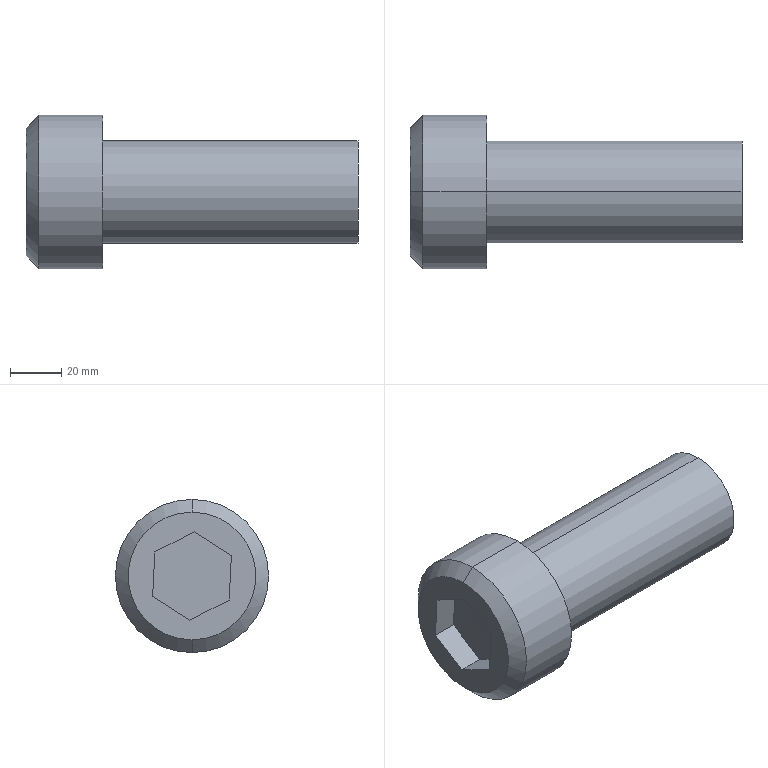Part | SolidWorks | features BaseBody 12, ICE 10, Chamfer 2 | 1 solid | 16 faces | box 130 x 60 x 60 mm | volume 200467 mm3 | plane 10 | cylinder 4 | cone 2 | commonest cylinder face diameters 40 x2 60 x2
STEP:
#1=CARTESIAN_POINT('',(548.124,-238.28,806.023));
#2=VERTEX_POINT('',#1);
#3=CARTESIAN_POINT('',(548.124,-238.28,846.023));
#4=VERTEX_POINT('',#3);
#5=CARTESIAN_POINT('',(548.124,-238.28,826.023));
#6=DIRECTION('',(1.,0.,0.));
#7=DIRECTION('',(0.,0.,-1.));
#8=AXIS2_PLACEMENT_3D('',#5,#6,#7);
#9=CIRCLE('',#8,20.);
#10=EDGE_CURVE('',#2,#4,#9,.T.);
#11=ORIENTED_EDGE('',*,*,#10,.F.);
#12=CARTESIAN_POINT('',(448.124,-238.28,806.023));
#13=VERTEX_POINT('',#12);
#14=CARTESIAN_POINT('',(548.124,-238.28,806.023));
#15=DIRECTION('',(-1.,0.,0.));
#16=VECTOR('',#15,1000.);
#17=LINE('',#14,#16);
#18=EDGE_CURVE('',#2,#13,#17,.T.);
#19=ORIENTED_EDGE('',*,*,#18,.T.);
#20=CARTESIAN_POINT('',(448.124,-238.28,846.023));
#21=VERTEX_POINT('',#20);
#22=CARTESIAN_POINT('',(448.124,-238.28,826.023));
#23=DIRECTION('',(1.,0.,0.));
#24=DIRECTION('',(0.,0.,-1.));
#25=AXIS2_PLACEMENT_3D('',#22,#23,#24);
#26=CIRCLE('',#25,20.);
#27=EDGE_CURVE('',#13,#21,#26,.T.);
#28=ORIENTED_EDGE('',*,*,#27,.T.);
#29=CARTESIAN_POINT('',(548.124,-238.28,846.023));
#30=DIRECTION('',(-1.,0.,0.));
#31=VECTOR('',#30,1000.);
#32=LINE('',#29,#31);
#33=EDGE_CURVE('',#4,#21,#32,.T.);
#34=ORIENTED_EDGE('',*,*,#33,.F.);
#35=EDGE_LOOP('',(#11,#19,#28,#34));
#36=FACE_OUTER_BOUND('',#35,.T.);
#37=CARTESIAN_POINT('',(548.124,-238.28,826.023));
#38=DIRECTION('',(-1.,0.,0.));
#39=DIRECTION('',(0.,0.,1.));
#40=AXIS2_PLACEMENT_3D('',#37,#38,#39);
#41=CYLINDRICAL_SURFACE('',#40,20.);
#42=ADVANCED_FACE('',(#36),#41,.T.);
#43=CARTESIAN_POINT('',(418.124,-238.28,851.023));
#44=VERTEX_POINT('',#43);
#45=CARTESIAN_POINT('',(418.124,-238.28,801.023));
#46=VERTEX_POINT('',#45);
#47=CARTESIAN_POINT('',(418.124,-238.28,826.023));
#48=DIRECTION('',(-1.,0.,0.));
#49=DIRECTION('',(0.,0.,1.));
#50=AXIS2_PLACEMENT_3D('',#47,#48,#49);
#51=CIRCLE('',#50,25.);
#52=EDGE_CURVE('',#44,#46,#51,.T.);
#53=ORIENTED_EDGE('',*,*,#52,.F.);
#54=CARTESIAN_POINT('',(423.124,-238.28,856.023));
#55=VERTEX_POINT('',#54);
#56=CARTESIAN_POINT('',(418.124,-238.28,851.023));
#57=DIRECTION('',(0.7071,0.,0.7071));
#58=VECTOR('',#57,1000.);
#59=LINE('',#56,#58);
#60=EDGE_CURVE('',#44,#55,#59,.T.);
#61=ORIENTED_EDGE('',*,*,#60,.T.);
#62=CARTESIAN_POINT('',(423.124,-238.28,796.023));
#63=VERTEX_POINT('',#62);
#64=CARTESIAN_POINT('',(423.124,-238.28,826.023));
#65=DIRECTION('',(1.,0.,0.));
#66=DIRECTION('',(0.,0.,1.));
#67=AXIS2_PLACEMENT_3D('',#64,#65,#66);
#68=CIRCLE('',#67,30.);
#69=EDGE_CURVE('',#63,#55,#68,.T.);
#70=ORIENTED_EDGE('',*,*,#69,.F.);
#71=CARTESIAN_POINT('',(418.124,-238.28,801.023));
#72=DIRECTION('',(0.7071,0.,-0.7071));
#73=VECTOR('',#72,1000.);
#74=LINE('',#71,#73);
#75=EDGE_CURVE('',#46,#63,#74,.T.);
#76=ORIENTED_EDGE('',*,*,#75,.F.);
#77=EDGE_LOOP('',(#53,#61,#70,#76));
#78=FACE_OUTER_BOUND('',#77,.T.);
#79=CARTESIAN_POINT('',(418.124,-238.28,826.023));
#80=DIRECTION('',(1.,0.,0.));
#81=DIRECTION('',(0.,0.,-1.));
#82=AXIS2_PLACEMENT_3D('',#79,#80,#81);
#83=CONICAL_SURFACE('',#82,25.,0.7854);
#84=ADVANCED_FACE('',(#78),#83,.T.);
#85=ORIENTED_EDGE('',*,*,#69,.T.);
#86=CARTESIAN_POINT('',(448.124,-238.28,856.023));
#87=VERTEX_POINT('',#86);
#88=CARTESIAN_POINT('',(418.124,-238.28,856.023));
#89=DIRECTION('',(1.,0.,0.));
#90=VECTOR('',#89,1000.);
#91=LINE('',#88,#90);
#92=EDGE_CURVE('',#55,#87,#91,.T.);
#93=ORIENTED_EDGE('',*,*,#92,.T.);
#94=CARTESIAN_POINT('',(448.124,-238.28,796.023));
#95=VERTEX_POINT('',#94);
#96=CARTESIAN_POINT('',(448.124,-238.28,826.023));
#97=DIRECTION('',(-1.,0.,0.));
#98=DIRECTION('',(0.,0.,1.));
#99=AXIS2_PLACEMENT_3D('',#96,#97,#98);
#100=CIRCLE('',#99,30.);
#101=EDGE_CURVE('',#87,#95,#100,.T.);
#102=ORIENTED_EDGE('',*,*,#101,.T.);
#103=CARTESIAN_POINT('',(418.124,-238.28,796.023));
#104=DIRECTION('',(1.,0.,0.));
#105=VECTOR('',#104,1000.);
#106=LINE('',#103,#105);
#107=EDGE_CURVE('',#63,#95,#106,.T.);
#108=ORIENTED_EDGE('',*,*,#107,.F.);
#109=EDGE_LOOP('',(#85,#93,#102,#108));
#110=FACE_OUTER_BOUND('',#109,.T.);
#111=CARTESIAN_POINT('',(418.124,-238.28,826.023));
#112=DIRECTION('',(1.,0.,0.));
#113=DIRECTION('',(0.,0.,-1.));
#114=AXIS2_PLACEMENT_3D('',#111,#112,#113);
#115=CYLINDRICAL_SURFACE('',#114,30.);
#116=ADVANCED_FACE('',(#110),#115,.T.);
#117=ORIENTED_EDGE('',*,*,#92,.F.);
#118=CARTESIAN_POINT('',(423.124,-238.28,826.023));
#119=DIRECTION('',(1.,0.,0.));
#120=DIRECTION('',(0.,0.,1.));
#121=AXIS2_PLACEMENT_3D('',#118,#119,#120);
#122=CIRCLE('',#121,30.);
#123=EDGE_CURVE('',#55,#63,#122,.T.);
#124=ORIENTED_EDGE('',*,*,#123,.T.);
#125=ORIENTED_EDGE('',*,*,#107,.T.);
#126=CARTESIAN_POINT('',(448.124,-238.28,826.023));
#127=DIRECTION('',(-1.,0.,0.));
#128=DIRECTION('',(0.,0.,1.));
#129=AXIS2_PLACEMENT_3D('',#126,#127,#128);
#130=CIRCLE('',#129,30.);
#131=EDGE_CURVE('',#95,#87,#130,.T.);
#132=ORIENTED_EDGE('',*,*,#131,.T.);
#133=EDGE_LOOP('',(#117,#124,#125,#132));
#134=FACE_OUTER_BOUND('',#133,.T.);
#135=CARTESIAN_POINT('',(418.124,-238.28,826.023));
#136=DIRECTION('',(1.,0.,0.));
#137=DIRECTION('',(0.,0.,-1.));
#138=AXIS2_PLACEMENT_3D('',#135,#136,#137);
#139=CYLINDRICAL_SURFACE('',#138,30.);
#140=ADVANCED_FACE('',(#134),#139,.T.);
#141=CARTESIAN_POINT('',(418.124,-238.28,826.023));
#142=DIRECTION('',(-1.,0.,0.));
#143=DIRECTION('',(0.,0.,1.));
#144=AXIS2_PLACEMENT_3D('',#141,#142,#143);
#145=CIRCLE('',#144,25.);
#146=EDGE_CURVE('',#46,#44,#145,.T.);
#147=ORIENTED_EDGE('',*,*,#146,.T.);
#148=ORIENTED_EDGE('',*,*,#52,.T.);
#149=EDGE_LOOP('',(#147,#148));
#150=FACE_OUTER_BOUND('',#149,.T.);
#151=CARTESIAN_POINT('',(418.124,-239.145,843.322));
#152=VERTEX_POINT('',#151);
#153=CARTESIAN_POINT('',(418.124,-223.731,835.42));
#154=VERTEX_POINT('',#153);
#155=CARTESIAN_POINT('',(418.124,-239.145,843.322));
#156=DIRECTION('',(0.,0.8899,-0.4562));
#157=VECTOR('',#156,1000.);
#158=LINE('',#155,#157);
#159=EDGE_CURVE('',#152,#154,#158,.T.);
#160=ORIENTED_EDGE('',*,*,#159,.F.);
#161=CARTESIAN_POINT('',(418.124,-253.694,833.924));
#162=VERTEX_POINT('',#161);
#163=CARTESIAN_POINT('',(418.124,-253.694,833.924));
#164=DIRECTION('',(0.,0.84,0.5426));
#165=VECTOR('',#164,1000.);
#166=LINE('',#163,#165);
#167=EDGE_CURVE('',#162,#152,#166,.T.);
#168=ORIENTED_EDGE('',*,*,#167,.F.);
#169=CARTESIAN_POINT('',(418.124,-252.83,816.625));
#170=VERTEX_POINT('',#169);
#171=CARTESIAN_POINT('',(418.124,-252.83,816.625));
#172=DIRECTION('',(0.,-0.04989,0.9988));
#173=VECTOR('',#172,1000.);
#174=LINE('',#171,#173);
#175=EDGE_CURVE('',#170,#162,#174,.T.);
#176=ORIENTED_EDGE('',*,*,#175,.F.);
#177=CARTESIAN_POINT('',(418.124,-237.416,808.724));
#178=VERTEX_POINT('',#177);
#179=CARTESIAN_POINT('',(418.124,-237.416,808.724));
#180=DIRECTION('',(0.,-0.8899,0.4562));
#181=VECTOR('',#180,1000.);
#182=LINE('',#179,#181);
#183=EDGE_CURVE('',#178,#170,#182,.T.);
#184=ORIENTED_EDGE('',*,*,#183,.F.);
#185=CARTESIAN_POINT('',(418.124,-222.867,818.122));
#186=VERTEX_POINT('',#185);
#187=CARTESIAN_POINT('',(418.124,-222.867,818.122));
#188=DIRECTION('',(0.,-0.84,-0.5426));
#189=VECTOR('',#188,1000.);
#190=LINE('',#187,#189);
#191=EDGE_CURVE('',#186,#178,#190,.T.);
#192=ORIENTED_EDGE('',*,*,#191,.F.);
#193=CARTESIAN_POINT('',(418.124,-223.731,835.42));
#194=DIRECTION('',(0.,0.04989,-0.9988));
#195=VECTOR('',#194,1000.);
#196=LINE('',#193,#195);
#197=EDGE_CURVE('',#154,#186,#196,.T.);
#198=ORIENTED_EDGE('',*,*,#197,.F.);
#199=EDGE_LOOP('',(#160,#168,#176,#184,#192,#198));
#200=FACE_BOUND('',#199,.T.);
#201=CARTESIAN_POINT('',(418.124,-238.28,826.023));
#202=DIRECTION('',(-1.,0.,0.));
#203=DIRECTION('',(0.,0.,1.));
#204=AXIS2_PLACEMENT_3D('',#201,#202,#203);
#205=PLANE('',#204);
#206=ADVANCED_FACE('',(#150,#200),#205,.T.);
#207=CARTESIAN_POINT('',(448.124,-238.28,826.023));
#208=DIRECTION('',(1.,0.,0.));
#209=DIRECTION('',(0.,0.,-1.));
#210=AXIS2_PLACEMENT_3D('',#207,#208,#209);
#211=CIRCLE('',#210,20.);
#212=EDGE_CURVE('',#21,#13,#211,.T.);
#213=ORIENTED_EDGE('',*,*,#212,.F.);
#214=ORIENTED_EDGE('',*,*,#27,.F.);
#215=EDGE_LOOP('',(#213,#214));
#216=FACE_BOUND('',#215,.T.);
#217=ORIENTED_EDGE('',*,*,#131,.F.);
#218=ORIENTED_EDGE('',*,*,#101,.F.);
#219=EDGE_LOOP('',(#217,#218));
#220=FACE_OUTER_BOUND('',#219,.T.);
#221=CARTESIAN_POINT('',(448.124,-238.28,826.023));
#222=DIRECTION('',(-1.,0.,0.));
#223=DIRECTION('',(0.,0.,1.));
#224=AXIS2_PLACEMENT_3D('',#221,#222,#223);
#225=PLANE('',#224);
#226=ADVANCED_FACE('',(#216,#220),#225,.F.);
#227=ORIENTED_EDGE('',*,*,#159,.T.);
#228=CARTESIAN_POINT('',(428.124,-223.731,835.42));
#229=VERTEX_POINT('',#228);
#230=CARTESIAN_POINT('',(428.124,-223.731,835.42));
#231=DIRECTION('',(-1.,0.,0.));
#232=VECTOR('',#231,1000.);
#233=LINE('',#230,#232);
#234=EDGE_CURVE('',#229,#154,#233,.T.);
#235=ORIENTED_EDGE('',*,*,#234,.F.);
#236=CARTESIAN_POINT('',(428.124,-239.145,843.322));
#237=VERTEX_POINT('',#236);
#238=CARTESIAN_POINT('',(428.124,-239.145,843.322));
#239=DIRECTION('',(0.,0.8899,-0.4562));
#240=VECTOR('',#239,1000.);
#241=LINE('',#238,#240);
#242=EDGE_CURVE('',#237,#229,#241,.T.);
#243=ORIENTED_EDGE('',*,*,#242,.F.);
#244=CARTESIAN_POINT('',(428.124,-239.145,843.322));
#245=DIRECTION('',(-1.,0.,0.));
#246=VECTOR('',#245,1000.);
#247=LINE('',#244,#246);
#248=EDGE_CURVE('',#237,#152,#247,.T.);
#249=ORIENTED_EDGE('',*,*,#248,.T.);
#250=EDGE_LOOP('',(#227,#235,#243,#249));
#251=FACE_OUTER_BOUND('',#250,.T.);
#252=CARTESIAN_POINT('',(428.124,-239.145,843.322));
#253=DIRECTION('',(0.,0.4562,0.8899));
#254=DIRECTION('',(0.,-0.8899,0.4562));
#255=AXIS2_PLACEMENT_3D('',#252,#253,#254);
#256=PLANE('',#255);
#257=ADVANCED_FACE('',(#251),#256,.F.);
#258=ORIENTED_EDGE('',*,*,#167,.T.);
#259=ORIENTED_EDGE('',*,*,#248,.F.);
#260=CARTESIAN_POINT('',(428.124,-253.694,833.924));
#261=VERTEX_POINT('',#260);
#262=CARTESIAN_POINT('',(428.124,-253.694,833.924));
#263=DIRECTION('',(0.,0.84,0.5426));
#264=VECTOR('',#263,1000.);
#265=LINE('',#262,#264);
#266=EDGE_CURVE('',#261,#237,#265,.T.);
#267=ORIENTED_EDGE('',*,*,#266,.F.);
#268=CARTESIAN_POINT('',(428.124,-253.694,833.924));
#269=DIRECTION('',(-1.,0.,0.));
#270=VECTOR('',#269,1000.);
#271=LINE('',#268,#270);
#272=EDGE_CURVE('',#261,#162,#271,.T.);
#273=ORIENTED_EDGE('',*,*,#272,.T.);
#274=EDGE_LOOP('',(#258,#259,#267,#273));
#275=FACE_OUTER_BOUND('',#274,.T.);
#276=CARTESIAN_POINT('',(428.124,-253.694,833.924));
#277=DIRECTION('',(0.,-0.5426,0.84));
#278=DIRECTION('',(0.,-0.84,-0.5426));
#279=AXIS2_PLACEMENT_3D('',#276,#277,#278);
#280=PLANE('',#279);
#281=ADVANCED_FACE('',(#275),#280,.F.);
#282=ORIENTED_EDGE('',*,*,#175,.T.);
#283=ORIENTED_EDGE('',*,*,#272,.F.);
#284=CARTESIAN_POINT('',(428.124,-252.83,816.625));
#285=VERTEX_POINT('',#284);
#286=CARTESIAN_POINT('',(428.124,-252.83,816.625));
#287=DIRECTION('',(0.,-0.04989,0.9988));
#288=VECTOR('',#287,1000.);
#289=LINE('',#286,#288);
#290=EDGE_CURVE('',#285,#261,#289,.T.);
#291=ORIENTED_EDGE('',*,*,#290,.F.);
#292=CARTESIAN_POINT('',(428.124,-252.83,816.625));
#293=DIRECTION('',(-1.,0.,0.));
#294=VECTOR('',#293,1000.);
#295=LINE('',#292,#294);
#296=EDGE_CURVE('',#285,#170,#295,.T.);
#297=ORIENTED_EDGE('',*,*,#296,.T.);
#298=EDGE_LOOP('',(#282,#283,#291,#297));
#299=FACE_OUTER_BOUND('',#298,.T.);
#300=CARTESIAN_POINT('',(428.124,-252.83,816.625));
#301=DIRECTION('',(0.,-0.9988,-0.04989));
#302=DIRECTION('',(0.,0.04989,-0.9988));
#303=AXIS2_PLACEMENT_3D('',#300,#301,#302);
#304=PLANE('',#303);
#305=ADVANCED_FACE('',(#299),#304,.F.);
#306=ORIENTED_EDGE('',*,*,#183,.T.);
#307=ORIENTED_EDGE('',*,*,#296,.F.);
#308=CARTESIAN_POINT('',(428.124,-237.416,808.724));
#309=VERTEX_POINT('',#308);
#310=CARTESIAN_POINT('',(428.124,-237.416,808.724));
#311=DIRECTION('',(0.,-0.8899,0.4562));
#312=VECTOR('',#311,1000.);
#313=LINE('',#310,#312);
#314=EDGE_CURVE('',#309,#285,#313,.T.);
#315=ORIENTED_EDGE('',*,*,#314,.F.);
#316=CARTESIAN_POINT('',(428.124,-237.416,808.724));
#317=DIRECTION('',(-1.,0.,0.));
#318=VECTOR('',#317,1000.);
#319=LINE('',#316,#318);
#320=EDGE_CURVE('',#309,#178,#319,.T.);
#321=ORIENTED_EDGE('',*,*,#320,.T.);
#322=EDGE_LOOP('',(#306,#307,#315,#321));
#323=FACE_OUTER_BOUND('',#322,.T.);
#324=CARTESIAN_POINT('',(428.124,-237.416,808.724));
#325=DIRECTION('',(0.,-0.4562,-0.8899));
#326=DIRECTION('',(0.,0.8899,-0.4562));
#327=AXIS2_PLACEMENT_3D('',#324,#325,#326);
#328=PLANE('',#327);
#329=ADVANCED_FACE('',(#323),#328,.F.);
#330=ORIENTED_EDGE('',*,*,#191,.T.);
#331=ORIENTED_EDGE('',*,*,#320,.F.);
#332=CARTESIAN_POINT('',(428.124,-222.867,818.122));
#333=VERTEX_POINT('',#332);
#334=CARTESIAN_POINT('',(428.124,-222.867,818.122));
#335=DIRECTION('',(0.,-0.84,-0.5426));
#336=VECTOR('',#335,1000.);
#337=LINE('',#334,#336);
#338=EDGE_CURVE('',#333,#309,#337,.T.);
#339=ORIENTED_EDGE('',*,*,#338,.F.);
#340=CARTESIAN_POINT('',(428.124,-222.867,818.122));
#341=DIRECTION('',(-1.,0.,0.));
#342=VECTOR('',#341,1000.);
#343=LINE('',#340,#342);
#344=EDGE_CURVE('',#333,#186,#343,.T.);
#345=ORIENTED_EDGE('',*,*,#344,.T.);
#346=EDGE_LOOP('',(#330,#331,#339,#345));
#347=FACE_OUTER_BOUND('',#346,.T.);
#348=CARTESIAN_POINT('',(428.124,-222.867,818.122));
#349=DIRECTION('',(0.,0.5426,-0.84));
#350=DIRECTION('',(0.,0.84,0.5426));
#351=AXIS2_PLACEMENT_3D('',#348,#349,#350);
#352=PLANE('',#351);
#353=ADVANCED_FACE('',(#347),#352,.F.);
#354=ORIENTED_EDGE('',*,*,#197,.T.);
#355=ORIENTED_EDGE('',*,*,#344,.F.);
#356=CARTESIAN_POINT('',(428.124,-223.731,835.42));
#357=DIRECTION('',(0.,0.04989,-0.9988));
#358=VECTOR('',#357,1000.);
#359=LINE('',#356,#358);
#360=EDGE_CURVE('',#229,#333,#359,.T.);
#361=ORIENTED_EDGE('',*,*,#360,.F.);
#362=ORIENTED_EDGE('',*,*,#234,.T.);
#363=EDGE_LOOP('',(#354,#355,#361,#362));
#364=FACE_OUTER_BOUND('',#363,.T.);
#365=CARTESIAN_POINT('',(428.124,-223.731,835.42));
#366=DIRECTION('',(0.,0.9988,0.04989));
#367=DIRECTION('',(0.,-0.04989,0.9988));
#368=AXIS2_PLACEMENT_3D('',#365,#366,#367);
#369=PLANE('',#368);
#370=ADVANCED_FACE('',(#364),#369,.F.);
#371=ORIENTED_EDGE('',*,*,#242,.T.);
#372=ORIENTED_EDGE('',*,*,#360,.T.);
#373=ORIENTED_EDGE('',*,*,#338,.T.);
#374=ORIENTED_EDGE('',*,*,#314,.T.);
#375=ORIENTED_EDGE('',*,*,#290,.T.);
#376=ORIENTED_EDGE('',*,*,#266,.T.);
#377=EDGE_LOOP('',(#371,#372,#373,#374,#375,#376));
#378=FACE_OUTER_BOUND('',#377,.T.);
#379=CARTESIAN_POINT('',(428.124,0.,0.));
#380=DIRECTION('',(-1.,0.,0.));
#381=DIRECTION('',(0.,0.,1.));
#382=AXIS2_PLACEMENT_3D('',#379,#380,#381);
#383=PLANE('',#382);
#384=ADVANCED_FACE('',(#378),#383,.T.);
#385=ORIENTED_EDGE('',*,*,#60,.F.);
#386=ORIENTED_EDGE('',*,*,#146,.F.);
#387=ORIENTED_EDGE('',*,*,#75,.T.);
#388=ORIENTED_EDGE('',*,*,#123,.F.);
#389=EDGE_LOOP('',(#385,#386,#387,#388));
#390=FACE_OUTER_BOUND('',#389,.T.);
#391=CARTESIAN_POINT('',(418.124,-238.28,826.023));
#392=DIRECTION('',(1.,0.,0.));
#393=DIRECTION('',(0.,0.,-1.));
#394=AXIS2_PLACEMENT_3D('',#391,#392,#393);
#395=CONICAL_SURFACE('',#394,25.,0.7854);
#396=ADVANCED_FACE('',(#390),#395,.T.);
#397=ORIENTED_EDGE('',*,*,#18,.F.);
#398=CARTESIAN_POINT('',(548.124,-238.28,826.023));
#399=DIRECTION('',(1.,0.,0.));
#400=DIRECTION('',(0.,0.,-1.));
#401=AXIS2_PLACEMENT_3D('',#398,#399,#400);
#402=CIRCLE('',#401,20.);
#403=EDGE_CURVE('',#4,#2,#402,.T.);
#404=ORIENTED_EDGE('',*,*,#403,.F.);
#405=ORIENTED_EDGE('',*,*,#33,.T.);
#406=ORIENTED_EDGE('',*,*,#212,.T.);
#407=EDGE_LOOP('',(#397,#404,#405,#406));
#408=FACE_OUTER_BOUND('',#407,.T.);
#409=CARTESIAN_POINT('',(548.124,-238.28,826.023));
#410=DIRECTION('',(-1.,0.,0.));
#411=DIRECTION('',(0.,0.,1.));
#412=AXIS2_PLACEMENT_3D('',#409,#410,#411);
#413=CYLINDRICAL_SURFACE('',#412,20.);
#414=ADVANCED_FACE('',(#408),#413,.T.);
#415=ORIENTED_EDGE('',*,*,#403,.T.);
#416=ORIENTED_EDGE('',*,*,#10,.T.);
#417=EDGE_LOOP('',(#415,#416));
#418=FACE_OUTER_BOUND('',#417,.T.);
#419=CARTESIAN_POINT('',(548.124,-238.28,826.023));
#420=DIRECTION('',(1.,0.,0.));
#421=DIRECTION('',(0.,0.,-1.));
#422=AXIS2_PLACEMENT_3D('',#419,#420,#421);
#423=PLANE('',#422);
#424=ADVANCED_FACE('',(#418),#423,.T.);
#425=CLOSED_SHELL('',(#42,#84,#116,#140,#206,#226,#257,#281,#305,#329,#353,#370,#384,#396,#414,#424));
#426=MANIFOLD_SOLID_BREP('',#425);
#427=CARTESIAN_POINT('',(0.,0.,0.));
#428=DIRECTION('',(0.,0.,1.));
#429=DIRECTION('',(1.,0.,0.));
#430=AXIS2_PLACEMENT_3D('',#427,#428,#429);
#431=(LENGTH_UNIT()NAMED_UNIT(*)SI_UNIT(.MILLI.,.METRE.));
#432=UNCERTAINTY_MEASURE_WITH_UNIT(LENGTH_MEASURE(0.00001),#431,'','');
#433=(NAMED_UNIT(*)PLANE_ANGLE_UNIT()SI_UNIT($,.RADIAN.));
#434=(NAMED_UNIT(*)SI_UNIT($,.STERADIAN.)SOLID_ANGLE_UNIT());
#435=(GEOMETRIC_REPRESENTATION_CONTEXT(3)GLOBAL_UNCERTAINTY_ASSIGNED_CONTEXT((#432))GLOBAL_UNIT_ASSIGNED_CONTEXT((#431,#433,#434))REPRESENTATION_CONTEXT('',''));
#436=ADVANCED_BREP_SHAPE_REPRESENTATION('',(#426,#430),#435);